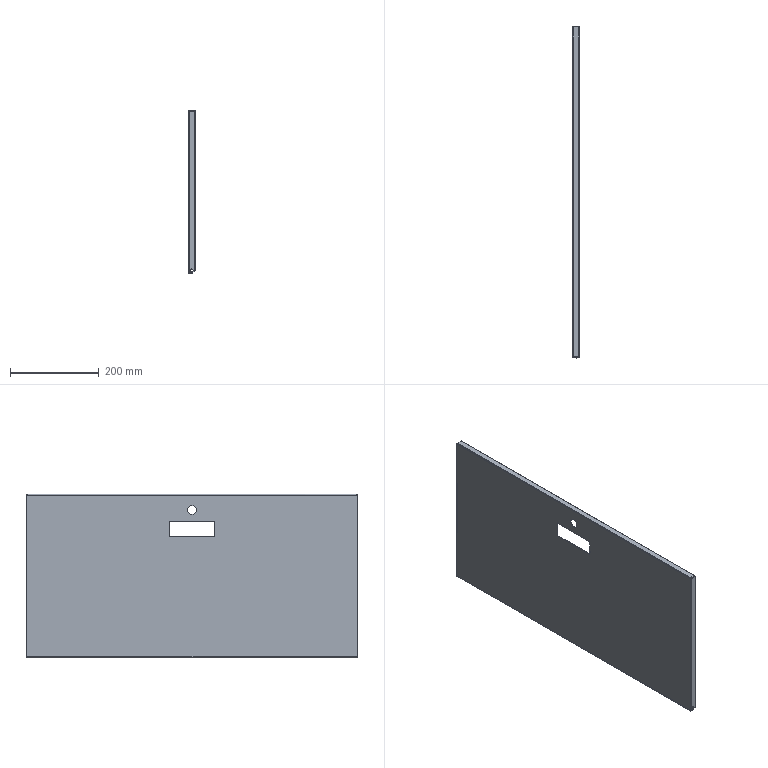Part | SolidWorks | features EdgeFlange 4, ICE 4, FlatPattern 1, SMBaseFlange 1, SheetMetal 1 | 1 solid | 92 faces | box 15 x 747 x 367.5 mm | volume 473438 mm3 | plane 62 | cylinder 22 | spline 8 | commonest cylinder face diameters 0.6 x7 3.6 x7 7 x4 20 x2 1.473 x1 4.473 x1